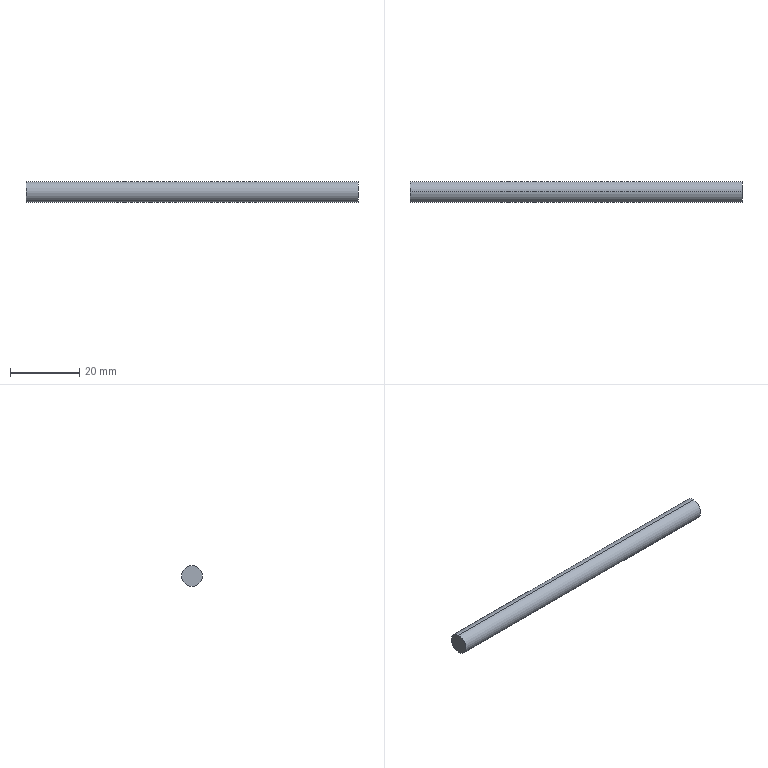Part | SolidWorks | features BaseBody 1 | 1 solid | 4 faces | box 96 x 6 x 6 mm | volume 2714 mm3 | cylinder 2 | plane 2 | commonest cylinder face diameters 6 x2
STEP:
#1=CARTESIAN_POINT('',(-48.,0.,-3.));
#2=VERTEX_POINT('',#1);
#3=CARTESIAN_POINT('',(-48.,0.,3.));
#4=VERTEX_POINT('',#3);
#5=CARTESIAN_POINT('',(-48.,0.,0.));
#6=DIRECTION('',(1.,0.,0.));
#7=DIRECTION('',(0.,0.,-1.));
#8=AXIS2_PLACEMENT_3D('',#5,#6,#7);
#9=CIRCLE('',#8,3.);
#10=EDGE_CURVE('',#2,#4,#9,.T.);
#11=ORIENTED_EDGE('',*,*,#10,.T.);
#12=CARTESIAN_POINT('',(48.,0.,3.));
#13=VERTEX_POINT('',#12);
#14=CARTESIAN_POINT('',(-48.,0.,3.));
#15=DIRECTION('',(1.,0.,0.));
#16=VECTOR('',#15,1000.);
#17=LINE('',#14,#16);
#18=EDGE_CURVE('',#4,#13,#17,.T.);
#19=ORIENTED_EDGE('',*,*,#18,.T.);
#20=CARTESIAN_POINT('',(48.,0.,-3.));
#21=VERTEX_POINT('',#20);
#22=CARTESIAN_POINT('',(48.,0.,0.));
#23=DIRECTION('',(-1.,0.,0.));
#24=DIRECTION('',(0.,0.,-1.));
#25=AXIS2_PLACEMENT_3D('',#22,#23,#24);
#26=CIRCLE('',#25,3.);
#27=EDGE_CURVE('',#13,#21,#26,.T.);
#28=ORIENTED_EDGE('',*,*,#27,.T.);
#29=CARTESIAN_POINT('',(-48.,0.,-3.));
#30=DIRECTION('',(1.,0.,0.));
#31=VECTOR('',#30,1000.);
#32=LINE('',#29,#31);
#33=EDGE_CURVE('',#2,#21,#32,.T.);
#34=ORIENTED_EDGE('',*,*,#33,.F.);
#35=EDGE_LOOP('',(#11,#19,#28,#34));
#36=FACE_OUTER_BOUND('',#35,.T.);
#37=CARTESIAN_POINT('',(-48.,0.,0.));
#38=DIRECTION('',(1.,0.,0.));
#39=DIRECTION('',(0.,0.,-1.));
#40=AXIS2_PLACEMENT_3D('',#37,#38,#39);
#41=CYLINDRICAL_SURFACE('',#40,3.);
#42=ADVANCED_FACE('',(#36),#41,.T.);
#43=ORIENTED_EDGE('',*,*,#18,.F.);
#44=CARTESIAN_POINT('',(-48.,0.,0.));
#45=DIRECTION('',(1.,0.,0.));
#46=DIRECTION('',(0.,0.,-1.));
#47=AXIS2_PLACEMENT_3D('',#44,#45,#46);
#48=CIRCLE('',#47,3.);
#49=EDGE_CURVE('',#4,#2,#48,.T.);
#50=ORIENTED_EDGE('',*,*,#49,.T.);
#51=ORIENTED_EDGE('',*,*,#33,.T.);
#52=CARTESIAN_POINT('',(48.,0.,0.));
#53=DIRECTION('',(-1.,0.,0.));
#54=DIRECTION('',(0.,0.,-1.));
#55=AXIS2_PLACEMENT_3D('',#52,#53,#54);
#56=CIRCLE('',#55,3.);
#57=EDGE_CURVE('',#21,#13,#56,.T.);
#58=ORIENTED_EDGE('',*,*,#57,.T.);
#59=EDGE_LOOP('',(#43,#50,#51,#58));
#60=FACE_OUTER_BOUND('',#59,.T.);
#61=CARTESIAN_POINT('',(-48.,0.,0.));
#62=DIRECTION('',(1.,0.,0.));
#63=DIRECTION('',(0.,0.,-1.));
#64=AXIS2_PLACEMENT_3D('',#61,#62,#63);
#65=CYLINDRICAL_SURFACE('',#64,3.);
#66=ADVANCED_FACE('',(#60),#65,.T.);
#67=ORIENTED_EDGE('',*,*,#10,.F.);
#68=ORIENTED_EDGE('',*,*,#49,.F.);
#69=EDGE_LOOP('',(#67,#68));
#70=FACE_OUTER_BOUND('',#69,.T.);
#71=CARTESIAN_POINT('',(-48.,0.,0.));
#72=DIRECTION('',(1.,0.,0.));
#73=DIRECTION('',(0.,0.,-1.));
#74=AXIS2_PLACEMENT_3D('',#71,#72,#73);
#75=PLANE('',#74);
#76=ADVANCED_FACE('',(#70),#75,.F.);
#77=ORIENTED_EDGE('',*,*,#57,.F.);
#78=ORIENTED_EDGE('',*,*,#27,.F.);
#79=EDGE_LOOP('',(#77,#78));
#80=FACE_OUTER_BOUND('',#79,.T.);
#81=CARTESIAN_POINT('',(48.,0.,0.));
#82=DIRECTION('',(1.,0.,0.));
#83=DIRECTION('',(0.,0.,-1.));
#84=AXIS2_PLACEMENT_3D('',#81,#82,#83);
#85=PLANE('',#84);
#86=ADVANCED_FACE('',(#80),#85,.T.);
#87=CLOSED_SHELL('',(#42,#66,#76,#86));
#88=MANIFOLD_SOLID_BREP('',#87);
#89=CARTESIAN_POINT('',(0.,0.,0.));
#90=DIRECTION('',(0.,0.,1.));
#91=DIRECTION('',(1.,0.,0.));
#92=AXIS2_PLACEMENT_3D('',#89,#90,#91);
#93=(LENGTH_UNIT()NAMED_UNIT(*)SI_UNIT(.MILLI.,.METRE.));
#94=UNCERTAINTY_MEASURE_WITH_UNIT(LENGTH_MEASURE(0.00001),#93,'','');
#95=(NAMED_UNIT(*)PLANE_ANGLE_UNIT()SI_UNIT($,.RADIAN.));
#96=(NAMED_UNIT(*)SI_UNIT($,.STERADIAN.)SOLID_ANGLE_UNIT());
#97=(GEOMETRIC_REPRESENTATION_CONTEXT(3)GLOBAL_UNCERTAINTY_ASSIGNED_CONTEXT((#94))GLOBAL_UNIT_ASSIGNED_CONTEXT((#93,#95,#96))REPRESENTATION_CONTEXT('',''));
#98=ADVANCED_BREP_SHAPE_REPRESENTATION('',(#88,#92),#97);